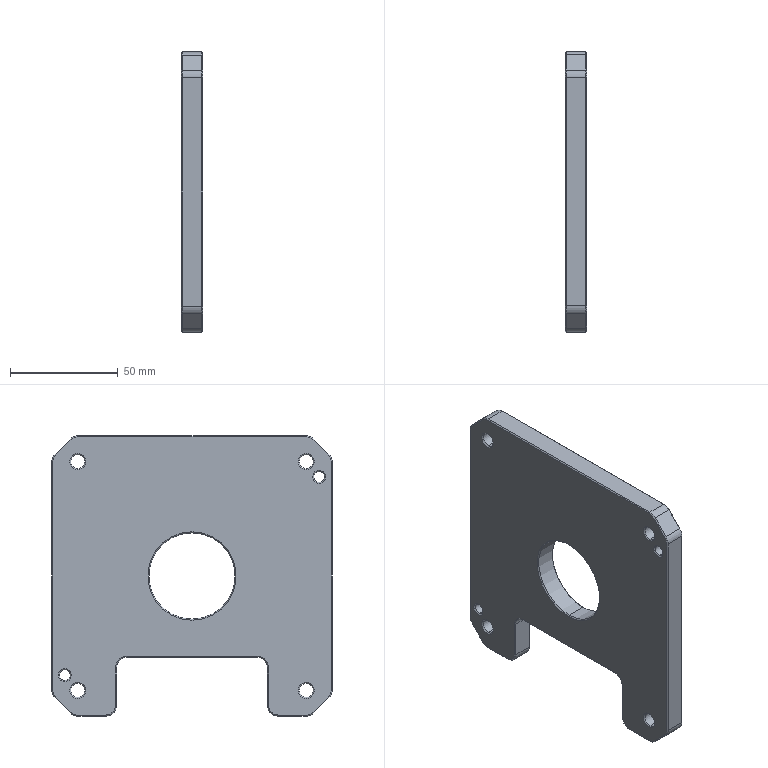Part | SolidWorks | features Cut 3, Chamfer 2, Fillet 2, Extrusion 1, ICE 1 | 1 solid | 116 faces | box 10 x 130 x 130 mm | volume 133322 mm3 | cone 52 | plane 38 | cylinder 26 | commonest cylinder face diameters 10 x12 6.5 x8 5 x4 40 x2